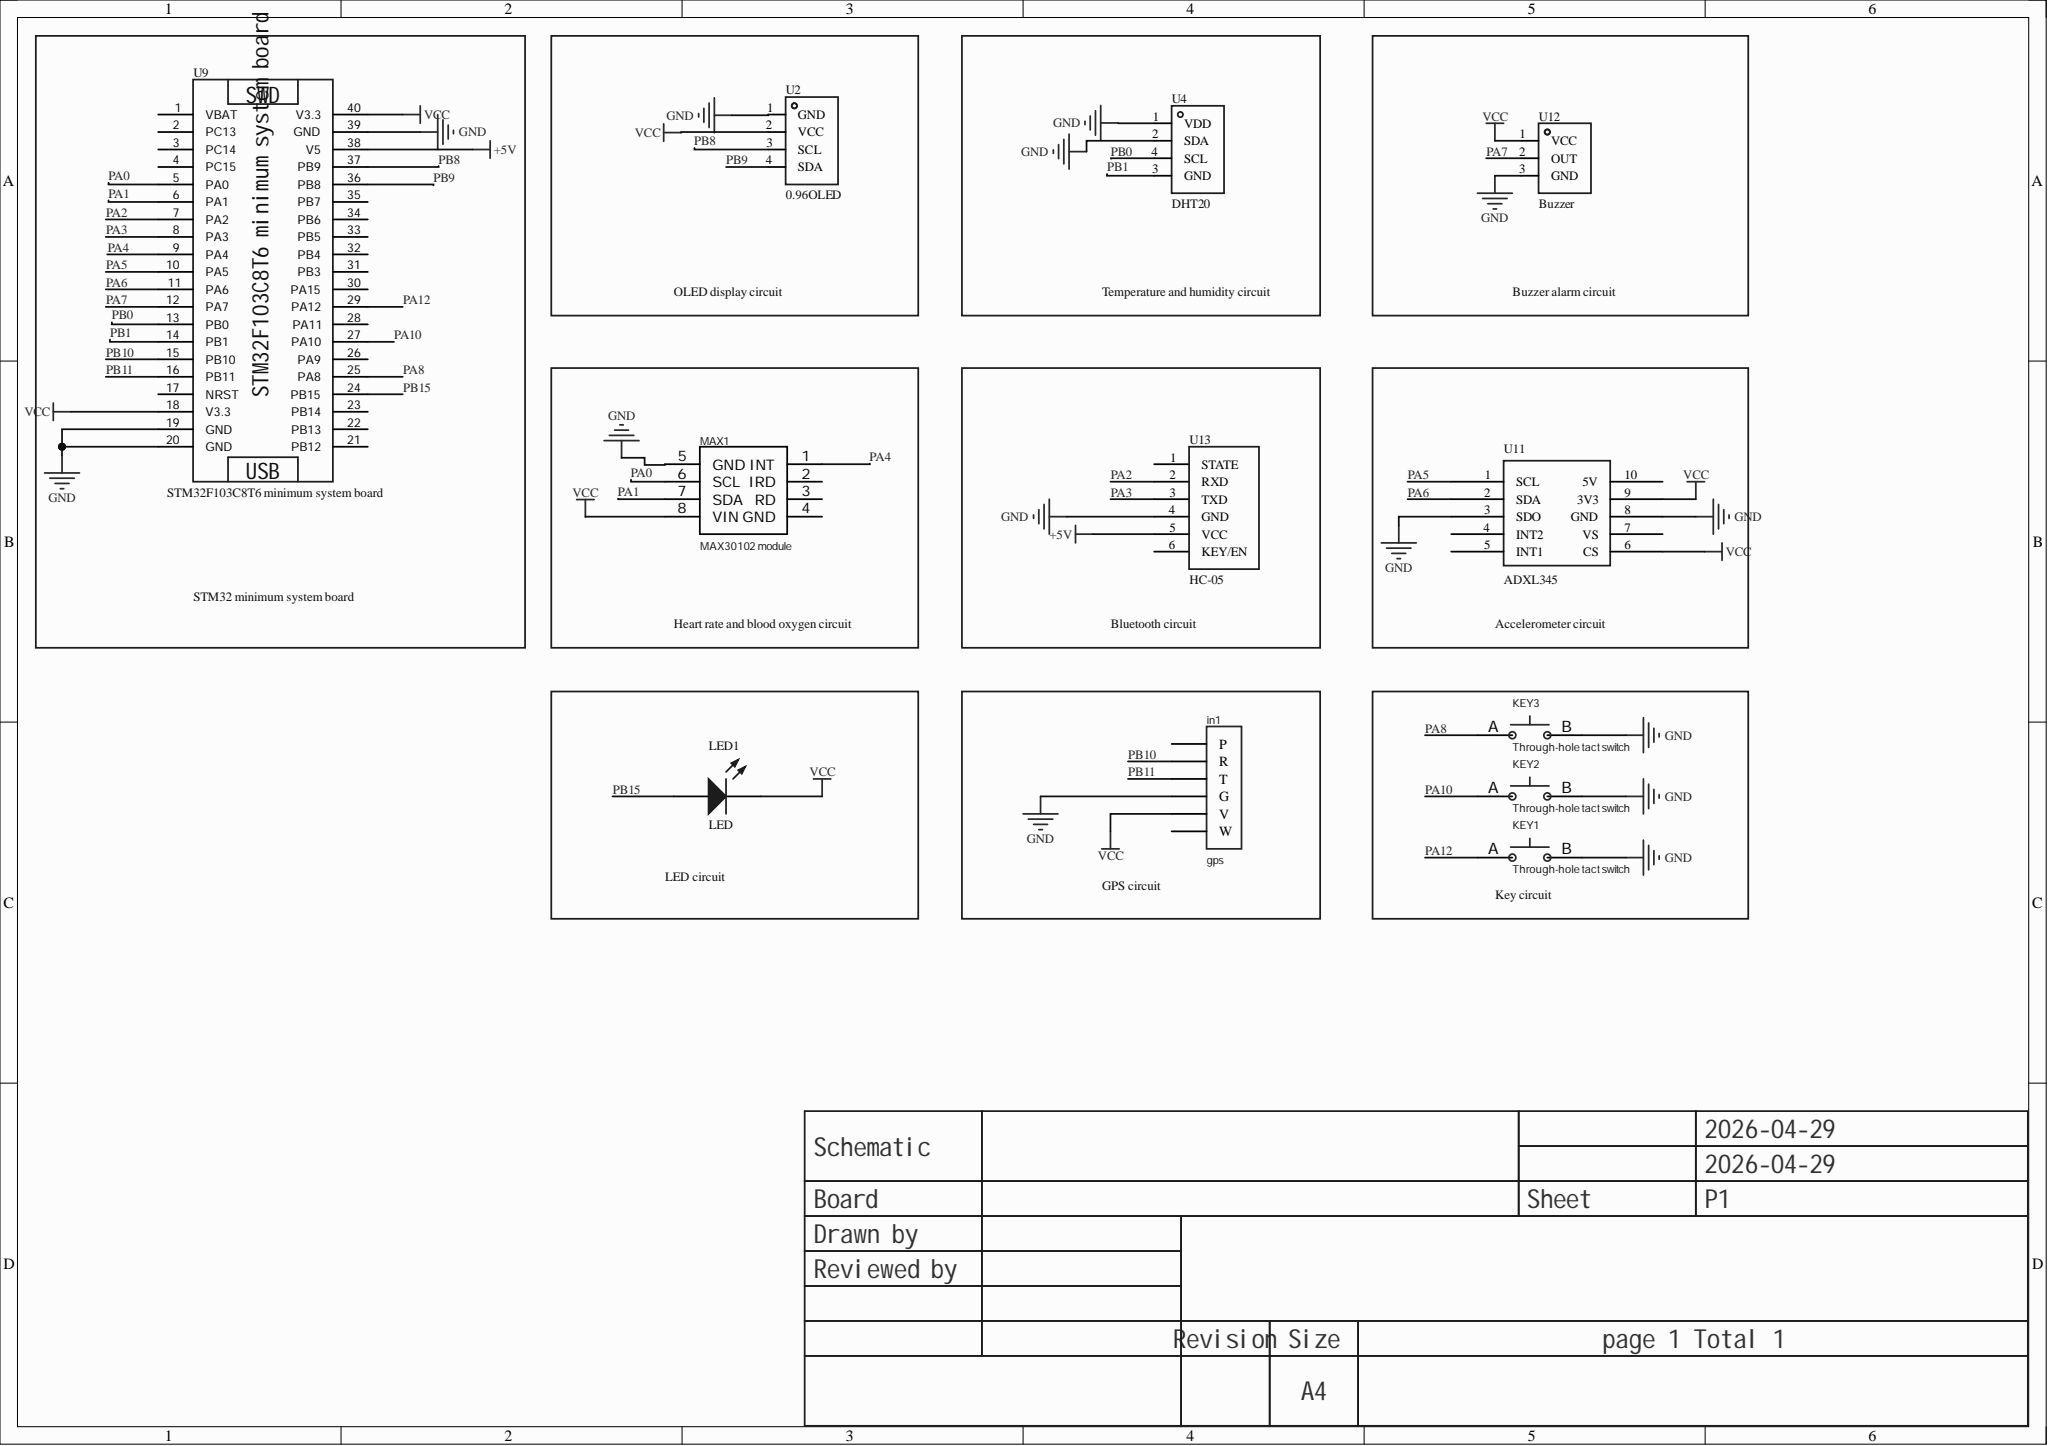Circuit board | Altium Designer | 12 parts | 21 nets
Bill of materials:
Comment,Description,Designator,Footprint,LibRef,Quantity
"gps","","in1","TYPE-C-6PIN-TH_C9900014686","6P","1"
"Through-hole tact switch","","KEY1, KEY2, KEY3","直插轻触开关3*6*5","直插轻触开关","3"
"LED","","LED1","HDR1X2","LED","1"
"MAX30102 module","","MAX1","COMM-SMD_8P-L20.2-W15.4-P2.54_MAX30102","MAX30102模块","1"
"0.96OLED","Core chip: SSD1315 chip; interface type: I2C; size (inch): 0.96; pixel resolution: 128x64;","U2","OLED-TH_L27.8-W27.2-P2.54_C9900033791","HS96L03W2C03","1"
"DHT20","DHT20是DHT11的全新升级产品，配置了专用的ASIC传感器芯片、高性能的半导体硅基电容式湿度传感器和一个标准的片上温度传感器，并使用了标准I²C数据输出信号格式。其性能已经大大提升，并且超过了前一代传感器（DHT11）的可靠性水平。新一代升级产品，经过改进使其在高温高湿环境下的性能更稳定；同时，产品的精度、响应时间、测量范围都得到了大幅的提升。","U4","SENSOR-TH_DHT20","DHT20","1"
"STM32F103C8T6 minimum system board","","U9","STM32F103C8T6核心板","STM32F103C8T6最小系统","1"
"ADXL345","","U11","COMM-TH_ADXL345","ADXL345","1"
"Buzzer","","U12","蜂鸣器","蜂鸣器","1"
"HC-05","","U13","HC05_6P","HC05","1"
Netlist (Protel format):
[
in1
TYPE-C-6PIN-TH_C9900014686
gps



]
[
KEY1
直插轻触开关3*6*5
Through-hole tact switch



]
[
KEY2
直插轻触开关3*6*5
Through-hole tact switch



]
[
KEY3
直插轻触开关3*6*5
Through-hole tact switch



]
[
LED1
HDR1X2
LED



]
[
MAX1
COMM-SMD_8P-L20.2-W15.4-P2.54_MAX30102
MAX30102 module



]
[
U2
OLED-TH_L27.8-W27.2-P2.54_C9900033791
0.96OLED



]
[
U4
SENSOR-TH_DHT20
DHT20



]
[
U9
STM32F103C8T6核心板
STM32F103C8T6 minimum system board



]
[
U11
COMM-TH_ADXL345
ADXL345



]
[
U12
蜂鸣器
Buzzer



]
[
U13
HC05_6P
HC-05



]
(
VCC
in1-5
LED1-2
U2-2
U9-18
U9-40
U11-6
U11-9
U12-1
)
(
PB15
LED1-1
U9-24
)
(
PB11
in1-3
U9-16
)
(
PB10
in1-2
U9-15
)
(
PB9
U2-4
U9-36
)
(
PB8
U2-3
U9-37
)
(
PB1
U4-3
U9-14
)
(
PB0
U4-4
U9-13
)
(
PA12
KEY1-A
U9-29
)
(
PA10
KEY2-A
U9-27
)
(
PA8
KEY3-A
U9-25
)
(
PA7
U9-12
U12-2
)
(
PA6
U9-11
U11-2
)
(
PA5
U9-10
U11-1
)
(
PA4
MAX1-1
U9-9
)
(
PA3
U9-8
U13-3
)
(
PA2
U9-7
U13-2
)
(
PA1
MAX1-7
U9-6
)
(
PA0
MAX1-6
U9-5
)
(
GND
in1-4
KEY1-B
KEY2-B
KEY3-B
U2-1
U4-2
U9-19
U9-20
U9-39
U11-3
U11-8
U12-3
U13-4
)
(
+5V
U9-38
U13-5
)